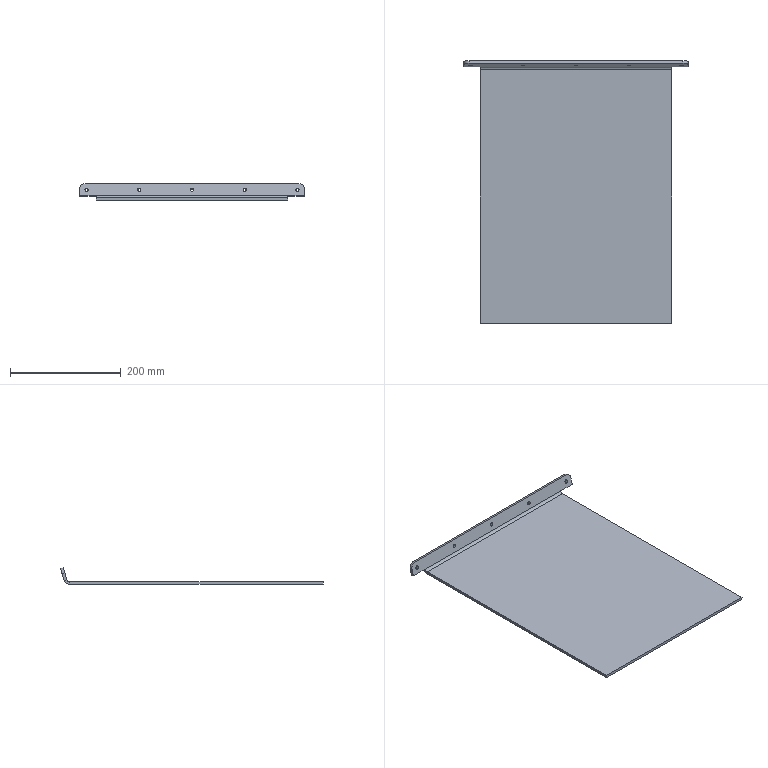Part | SolidWorks | features 3DProfileFeature 1, EdgeFlange 1, Fillet 1, FlatPattern 1, HoleWzd 1, SMBaseFlange 1, SheetMetal 1 | 1 solid | 38 faces | box 405 x 473.792 x 30.148 mm | volume 850700 mm3 | cylinder 14 | plane 14 | cone 10 | commonest cylinder face diameters 6 x10 20 x3 10 x1
STEP:
#1=CARTESIAN_POINT('',(-190.,237.073,15.005));
#2=VERTEX_POINT('',#1);
#3=CARTESIAN_POINT('',(-190.,238.832,20.741));
#4=VERTEX_POINT('',#3);
#5=CARTESIAN_POINT('',(-190.,237.952,17.873));
#6=DIRECTION('',(0.,0.9561,-0.2931));
#7=DIRECTION('',(0.,0.2931,0.9561));
#8=AXIS2_PLACEMENT_3D('',#5,#6,#7);
#9=CIRCLE('',#8,3.);
#10=EDGE_CURVE('',#2,#4,#9,.T.);
#11=ORIENTED_EDGE('',*,*,#10,.F.);
#12=CARTESIAN_POINT('',(-190.,237.09,14.974));
#13=VERTEX_POINT('',#12);
#14=CARTESIAN_POINT('',(-190.,237.09,14.974));
#15=DIRECTION('',(0.,0.4688,-0.8833));
#16=VECTOR('',#15,1000.);
#17=LINE('',#14,#16);
#18=EDGE_CURVE('',#2,#13,#17,.T.);
#19=ORIENTED_EDGE('',*,*,#18,.T.);
#20=CARTESIAN_POINT('',(-190.,238.863,20.758));
#21=VERTEX_POINT('',#20);
#22=CARTESIAN_POINT('',(-190.,237.976,17.866));
#23=DIRECTION('',(0.,0.9561,-0.2931));
#24=DIRECTION('',(0.,0.2931,0.9561));
#25=AXIS2_PLACEMENT_3D('',#22,#23,#24);
#26=CIRCLE('',#25,3.025);
#27=EDGE_CURVE('',#13,#21,#26,.T.);
#28=ORIENTED_EDGE('',*,*,#27,.T.);
#29=CARTESIAN_POINT('',(-190.,238.863,20.758));
#30=DIRECTION('',(0.,0.8833,0.4688));
#31=VECTOR('',#30,1000.);
#32=LINE('',#29,#31);
#33=EDGE_CURVE('',#4,#21,#32,.T.);
#34=ORIENTED_EDGE('',*,*,#33,.F.);
#35=EDGE_LOOP('',(#11,#19,#28,#34));
#36=FACE_OUTER_BOUND('',#35,.T.);
#37=CARTESIAN_POINT('',(-190.,237.976,17.866));
#38=DIRECTION('',(0.,0.9561,-0.2931));
#39=DIRECTION('',(0.,0.2931,0.9561));
#40=AXIS2_PLACEMENT_3D('',#37,#38,#39);
#41=CONICAL_SURFACE('',#40,3.025,0.7854);
#42=ADVANCED_FACE('',(#36),#41,.F.);
#43=CARTESIAN_POINT('',(-190.,232.317,16.463));
#44=VERTEX_POINT('',#43);
#45=CARTESIAN_POINT('',(-190.,234.075,22.199));
#46=VERTEX_POINT('',#45);
#47=CARTESIAN_POINT('',(-190.,233.196,19.331));
#48=DIRECTION('',(0.,0.9561,-0.2931));
#49=DIRECTION('',(0.,0.2931,0.9561));
#50=AXIS2_PLACEMENT_3D('',#47,#48,#49);
#51=CIRCLE('',#50,3.);
#52=EDGE_CURVE('',#44,#46,#51,.T.);
#53=ORIENTED_EDGE('',*,*,#52,.F.);
#54=CARTESIAN_POINT('',(-190.,237.097,14.998));
#55=DIRECTION('',(0.,0.9561,-0.2931));
#56=VECTOR('',#55,1000.);
#57=LINE('',#54,#56);
#58=EDGE_CURVE('',#44,#2,#57,.T.);
#59=ORIENTED_EDGE('',*,*,#58,.T.);
#60=ORIENTED_EDGE('',*,*,#10,.T.);
#61=CARTESIAN_POINT('',(-190.,238.855,20.734));
#62=DIRECTION('',(0.,0.9561,-0.2931));
#63=VECTOR('',#62,1000.);
#64=LINE('',#61,#63);
#65=EDGE_CURVE('',#46,#4,#64,.T.);
#66=ORIENTED_EDGE('',*,*,#65,.F.);
#67=EDGE_LOOP('',(#53,#59,#60,#66));
#68=FACE_OUTER_BOUND('',#67,.T.);
#69=CARTESIAN_POINT('',(-190.,237.976,17.866));
#70=DIRECTION('',(0.,0.9561,-0.2931));
#71=DIRECTION('',(0.,0.2931,0.9561));
#72=AXIS2_PLACEMENT_3D('',#69,#70,#71);
#73=CYLINDRICAL_SURFACE('',#72,3.);
#74=ADVANCED_FACE('',(#68),#73,.F.);
#75=CARTESIAN_POINT('',(-95.,237.073,15.005));
#76=VERTEX_POINT('',#75);
#77=CARTESIAN_POINT('',(-95.,238.832,20.741));
#78=VERTEX_POINT('',#77);
#79=CARTESIAN_POINT('',(-95.,237.952,17.873));
#80=DIRECTION('',(0.,0.9561,-0.2931));
#81=DIRECTION('',(0.,0.2931,0.9561));
#82=AXIS2_PLACEMENT_3D('',#79,#80,#81);
#83=CIRCLE('',#82,3.);
#84=EDGE_CURVE('',#76,#78,#83,.T.);
#85=ORIENTED_EDGE('',*,*,#84,.F.);
#86=CARTESIAN_POINT('',(-95.,237.09,14.974));
#87=VERTEX_POINT('',#86);
#88=CARTESIAN_POINT('',(-95.,237.09,14.974));
#89=DIRECTION('',(0.,0.4688,-0.8833));
#90=VECTOR('',#89,1000.);
#91=LINE('',#88,#90);
#92=EDGE_CURVE('',#76,#87,#91,.T.);
#93=ORIENTED_EDGE('',*,*,#92,.T.);
#94=CARTESIAN_POINT('',(-95.,238.863,20.758));
#95=VERTEX_POINT('',#94);
#96=CARTESIAN_POINT('',(-95.,237.976,17.866));
#97=DIRECTION('',(0.,0.9561,-0.2931));
#98=DIRECTION('',(0.,0.2931,0.9561));
#99=AXIS2_PLACEMENT_3D('',#96,#97,#98);
#100=CIRCLE('',#99,3.025);
#101=EDGE_CURVE('',#87,#95,#100,.T.);
#102=ORIENTED_EDGE('',*,*,#101,.T.);
#103=CARTESIAN_POINT('',(-95.,238.863,20.758));
#104=DIRECTION('',(0.,0.8833,0.4688));
#105=VECTOR('',#104,1000.);
#106=LINE('',#103,#105);
#107=EDGE_CURVE('',#78,#95,#106,.T.);
#108=ORIENTED_EDGE('',*,*,#107,.F.);
#109=EDGE_LOOP('',(#85,#93,#102,#108));
#110=FACE_OUTER_BOUND('',#109,.T.);
#111=CARTESIAN_POINT('',(-95.,237.976,17.866));
#112=DIRECTION('',(0.,0.9561,-0.2931));
#113=DIRECTION('',(0.,0.2931,0.9561));
#114=AXIS2_PLACEMENT_3D('',#111,#112,#113);
#115=CONICAL_SURFACE('',#114,3.025,0.7854);
#116=ADVANCED_FACE('',(#110),#115,.F.);
#117=CARTESIAN_POINT('',(-95.,232.317,16.463));
#118=VERTEX_POINT('',#117);
#119=CARTESIAN_POINT('',(-95.,234.075,22.199));
#120=VERTEX_POINT('',#119);
#121=CARTESIAN_POINT('',(-95.,233.196,19.331));
#122=DIRECTION('',(0.,0.9561,-0.2931));
#123=DIRECTION('',(0.,0.2931,0.9561));
#124=AXIS2_PLACEMENT_3D('',#121,#122,#123);
#125=CIRCLE('',#124,3.);
#126=EDGE_CURVE('',#118,#120,#125,.T.);
#127=ORIENTED_EDGE('',*,*,#126,.F.);
#128=CARTESIAN_POINT('',(-95.,237.097,14.998));
#129=DIRECTION('',(0.,0.9561,-0.2931));
#130=VECTOR('',#129,1000.);
#131=LINE('',#128,#130);
#132=EDGE_CURVE('',#118,#76,#131,.T.);
#133=ORIENTED_EDGE('',*,*,#132,.T.);
#134=ORIENTED_EDGE('',*,*,#84,.T.);
#135=CARTESIAN_POINT('',(-95.,238.855,20.734));
#136=DIRECTION('',(0.,0.9561,-0.2931));
#137=VECTOR('',#136,1000.);
#138=LINE('',#135,#137);
#139=EDGE_CURVE('',#120,#78,#138,.T.);
#140=ORIENTED_EDGE('',*,*,#139,.F.);
#141=EDGE_LOOP('',(#127,#133,#134,#140));
#142=FACE_OUTER_BOUND('',#141,.T.);
#143=CARTESIAN_POINT('',(-95.,237.976,17.866));
#144=DIRECTION('',(0.,0.9561,-0.2931));
#145=DIRECTION('',(0.,0.2931,0.9561));
#146=AXIS2_PLACEMENT_3D('',#143,#144,#145);
#147=CYLINDRICAL_SURFACE('',#146,3.);
#148=ADVANCED_FACE('',(#142),#147,.F.);
#149=CARTESIAN_POINT('',(0.,237.073,15.005));
#150=VERTEX_POINT('',#149);
#151=CARTESIAN_POINT('',(0.,238.832,20.741));
#152=VERTEX_POINT('',#151);
#153=CARTESIAN_POINT('',(0.,237.952,17.873));
#154=DIRECTION('',(0.,0.9561,-0.2931));
#155=DIRECTION('',(0.,0.2931,0.9561));
#156=AXIS2_PLACEMENT_3D('',#153,#154,#155);
#157=CIRCLE('',#156,3.);
#158=EDGE_CURVE('',#150,#152,#157,.T.);
#159=ORIENTED_EDGE('',*,*,#158,.F.);
#160=CARTESIAN_POINT('',(0.,237.09,14.974));
#161=VERTEX_POINT('',#160);
#162=CARTESIAN_POINT('',(0.,237.09,14.974));
#163=DIRECTION('',(0.,0.4688,-0.8833));
#164=VECTOR('',#163,1000.);
#165=LINE('',#162,#164);
#166=EDGE_CURVE('',#150,#161,#165,.T.);
#167=ORIENTED_EDGE('',*,*,#166,.T.);
#168=CARTESIAN_POINT('',(0.,238.863,20.758));
#169=VERTEX_POINT('',#168);
#170=CARTESIAN_POINT('',(0.,237.976,17.866));
#171=DIRECTION('',(0.,0.9561,-0.2931));
#172=DIRECTION('',(0.,0.2931,0.9561));
#173=AXIS2_PLACEMENT_3D('',#170,#171,#172);
#174=CIRCLE('',#173,3.025);
#175=EDGE_CURVE('',#161,#169,#174,.T.);
#176=ORIENTED_EDGE('',*,*,#175,.T.);
#177=CARTESIAN_POINT('',(0.,238.863,20.758));
#178=DIRECTION('',(0.,0.8833,0.4688));
#179=VECTOR('',#178,1000.);
#180=LINE('',#177,#179);
#181=EDGE_CURVE('',#152,#169,#180,.T.);
#182=ORIENTED_EDGE('',*,*,#181,.F.);
#183=EDGE_LOOP('',(#159,#167,#176,#182));
#184=FACE_OUTER_BOUND('',#183,.T.);
#185=CARTESIAN_POINT('',(0.,237.976,17.866));
#186=DIRECTION('',(0.,0.9561,-0.2931));
#187=DIRECTION('',(0.,0.2931,0.9561));
#188=AXIS2_PLACEMENT_3D('',#185,#186,#187);
#189=CONICAL_SURFACE('',#188,3.025,0.7854);
#190=ADVANCED_FACE('',(#184),#189,.F.);
#191=CARTESIAN_POINT('',(0.,232.317,16.463));
#192=VERTEX_POINT('',#191);
#193=CARTESIAN_POINT('',(0.,234.075,22.199));
#194=VERTEX_POINT('',#193);
#195=CARTESIAN_POINT('',(0.,233.196,19.331));
#196=DIRECTION('',(0.,0.9561,-0.2931));
#197=DIRECTION('',(0.,0.2931,0.9561));
#198=AXIS2_PLACEMENT_3D('',#195,#196,#197);
#199=CIRCLE('',#198,3.);
#200=EDGE_CURVE('',#192,#194,#199,.T.);
#201=ORIENTED_EDGE('',*,*,#200,.F.);
#202=CARTESIAN_POINT('',(0.,237.097,14.998));
#203=DIRECTION('',(0.,0.9561,-0.2931));
#204=VECTOR('',#203,1000.);
#205=LINE('',#202,#204);
#206=EDGE_CURVE('',#192,#150,#205,.T.);
#207=ORIENTED_EDGE('',*,*,#206,.T.);
#208=ORIENTED_EDGE('',*,*,#158,.T.);
#209=CARTESIAN_POINT('',(0.,238.855,20.734));
#210=DIRECTION('',(0.,0.9561,-0.2931));
#211=VECTOR('',#210,1000.);
#212=LINE('',#209,#211);
#213=EDGE_CURVE('',#194,#152,#212,.T.);
#214=ORIENTED_EDGE('',*,*,#213,.F.);
#215=EDGE_LOOP('',(#201,#207,#208,#214));
#216=FACE_OUTER_BOUND('',#215,.T.);
#217=CARTESIAN_POINT('',(0.,237.976,17.866));
#218=DIRECTION('',(0.,0.9561,-0.2931));
#219=DIRECTION('',(0.,0.2931,0.9561));
#220=AXIS2_PLACEMENT_3D('',#217,#218,#219);
#221=CYLINDRICAL_SURFACE('',#220,3.);
#222=ADVANCED_FACE('',(#216),#221,.F.);
#223=CARTESIAN_POINT('',(95.,237.073,15.005));
#224=VERTEX_POINT('',#223);
#225=CARTESIAN_POINT('',(95.,238.832,20.741));
#226=VERTEX_POINT('',#225);
#227=CARTESIAN_POINT('',(95.,237.952,17.873));
#228=DIRECTION('',(0.,0.9561,-0.2931));
#229=DIRECTION('',(0.,0.2931,0.9561));
#230=AXIS2_PLACEMENT_3D('',#227,#228,#229);
#231=CIRCLE('',#230,3.);
#232=EDGE_CURVE('',#224,#226,#231,.T.);
#233=ORIENTED_EDGE('',*,*,#232,.F.);
#234=CARTESIAN_POINT('',(95.,237.09,14.974));
#235=VERTEX_POINT('',#234);
#236=CARTESIAN_POINT('',(95.,237.09,14.974));
#237=DIRECTION('',(0.,0.4688,-0.8833));
#238=VECTOR('',#237,1000.);
#239=LINE('',#236,#238);
#240=EDGE_CURVE('',#224,#235,#239,.T.);
#241=ORIENTED_EDGE('',*,*,#240,.T.);
#242=CARTESIAN_POINT('',(95.,238.863,20.758));
#243=VERTEX_POINT('',#242);
#244=CARTESIAN_POINT('',(95.,237.976,17.866));
#245=DIRECTION('',(0.,0.9561,-0.2931));
#246=DIRECTION('',(0.,0.2931,0.9561));
#247=AXIS2_PLACEMENT_3D('',#244,#245,#246);
#248=CIRCLE('',#247,3.025);
#249=EDGE_CURVE('',#235,#243,#248,.T.);
#250=ORIENTED_EDGE('',*,*,#249,.T.);
#251=CARTESIAN_POINT('',(95.,238.863,20.758));
#252=DIRECTION('',(0.,0.8833,0.4688));
#253=VECTOR('',#252,1000.);
#254=LINE('',#251,#253);
#255=EDGE_CURVE('',#226,#243,#254,.T.);
#256=ORIENTED_EDGE('',*,*,#255,.F.);
#257=EDGE_LOOP('',(#233,#241,#250,#256));
#258=FACE_OUTER_BOUND('',#257,.T.);
#259=CARTESIAN_POINT('',(95.,237.976,17.866));
#260=DIRECTION('',(0.,0.9561,-0.2931));
#261=DIRECTION('',(0.,0.2931,0.9561));
#262=AXIS2_PLACEMENT_3D('',#259,#260,#261);
#263=CONICAL_SURFACE('',#262,3.025,0.7854);
#264=ADVANCED_FACE('',(#258),#263,.F.);
#265=CARTESIAN_POINT('',(95.,232.317,16.463));
#266=VERTEX_POINT('',#265);
#267=CARTESIAN_POINT('',(95.,234.075,22.199));
#268=VERTEX_POINT('',#267);
#269=CARTESIAN_POINT('',(95.,233.196,19.331));
#270=DIRECTION('',(0.,0.9561,-0.2931));
#271=DIRECTION('',(0.,0.2931,0.9561));
#272=AXIS2_PLACEMENT_3D('',#269,#270,#271);
#273=CIRCLE('',#272,3.);
#274=EDGE_CURVE('',#266,#268,#273,.T.);
#275=ORIENTED_EDGE('',*,*,#274,.F.);
#276=CARTESIAN_POINT('',(95.,237.097,14.998));
#277=DIRECTION('',(0.,0.9561,-0.2931));
#278=VECTOR('',#277,1000.);
#279=LINE('',#276,#278);
#280=EDGE_CURVE('',#266,#224,#279,.T.);
#281=ORIENTED_EDGE('',*,*,#280,.T.);
#282=ORIENTED_EDGE('',*,*,#232,.T.);
#283=CARTESIAN_POINT('',(95.,238.855,20.734));
#284=DIRECTION('',(0.,0.9561,-0.2931));
#285=VECTOR('',#284,1000.);
#286=LINE('',#283,#285);
#287=EDGE_CURVE('',#268,#226,#286,.T.);
#288=ORIENTED_EDGE('',*,*,#287,.F.);
#289=EDGE_LOOP('',(#275,#281,#282,#288));
#290=FACE_OUTER_BOUND('',#289,.T.);
#291=CARTESIAN_POINT('',(95.,237.976,17.866));
#292=DIRECTION('',(0.,0.9561,-0.2931));
#293=DIRECTION('',(0.,0.2931,0.9561));
#294=AXIS2_PLACEMENT_3D('',#291,#292,#293);
#295=CYLINDRICAL_SURFACE('',#294,3.);
#296=ADVANCED_FACE('',(#290),#295,.F.);
#297=CARTESIAN_POINT('',(190.,237.073,15.005));
#298=VERTEX_POINT('',#297);
#299=CARTESIAN_POINT('',(190.,238.832,20.741));
#300=VERTEX_POINT('',#299);
#301=CARTESIAN_POINT('',(190.,237.952,17.873));
#302=DIRECTION('',(0.,0.9561,-0.2931));
#303=DIRECTION('',(0.,0.2931,0.9561));
#304=AXIS2_PLACEMENT_3D('',#301,#302,#303);
#305=CIRCLE('',#304,3.);
#306=EDGE_CURVE('',#298,#300,#305,.T.);
#307=ORIENTED_EDGE('',*,*,#306,.F.);
#308=CARTESIAN_POINT('',(190.,237.09,14.974));
#309=VERTEX_POINT('',#308);
#310=CARTESIAN_POINT('',(190.,237.09,14.974));
#311=DIRECTION('',(0.,0.4688,-0.8833));
#312=VECTOR('',#311,1000.);
#313=LINE('',#310,#312);
#314=EDGE_CURVE('',#298,#309,#313,.T.);
#315=ORIENTED_EDGE('',*,*,#314,.T.);
#316=CARTESIAN_POINT('',(190.,238.863,20.758));
#317=VERTEX_POINT('',#316);
#318=CARTESIAN_POINT('',(190.,237.976,17.866));
#319=DIRECTION('',(0.,0.9561,-0.2931));
#320=DIRECTION('',(0.,0.2931,0.9561));
#321=AXIS2_PLACEMENT_3D('',#318,#319,#320);
#322=CIRCLE('',#321,3.025);
#323=EDGE_CURVE('',#309,#317,#322,.T.);
#324=ORIENTED_EDGE('',*,*,#323,.T.);
#325=CARTESIAN_POINT('',(190.,238.863,20.758));
#326=DIRECTION('',(0.,0.8833,0.4688));
#327=VECTOR('',#326,1000.);
#328=LINE('',#325,#327);
#329=EDGE_CURVE('',#300,#317,#328,.T.);
#330=ORIENTED_EDGE('',*,*,#329,.F.);
#331=EDGE_LOOP('',(#307,#315,#324,#330));
#332=FACE_OUTER_BOUND('',#331,.T.);
#333=CARTESIAN_POINT('',(190.,237.976,17.866));
#334=DIRECTION('',(0.,0.9561,-0.2931));
#335=DIRECTION('',(0.,0.2931,0.9561));
#336=AXIS2_PLACEMENT_3D('',#333,#334,#335);
#337=CONICAL_SURFACE('',#336,3.025,0.7854);
#338=ADVANCED_FACE('',(#332),#337,.F.);
#339=CARTESIAN_POINT('',(190.,232.317,16.463));
#340=VERTEX_POINT('',#339);
#341=CARTESIAN_POINT('',(190.,234.075,22.199));
#342=VERTEX_POINT('',#341);
#343=CARTESIAN_POINT('',(190.,233.196,19.331));
#344=DIRECTION('',(0.,0.9561,-0.2931));
#345=DIRECTION('',(0.,0.2931,0.9561));
#346=AXIS2_PLACEMENT_3D('',#343,#344,#345);
#347=CIRCLE('',#346,3.);
#348=EDGE_CURVE('',#340,#342,#347,.T.);
#349=ORIENTED_EDGE('',*,*,#348,.F.);
#350=CARTESIAN_POINT('',(190.,237.097,14.998));
#351=DIRECTION('',(0.,0.9561,-0.2931));
#352=VECTOR('',#351,1000.);
#353=LINE('',#350,#352);
#354=EDGE_CURVE('',#340,#298,#353,.T.);
#355=ORIENTED_EDGE('',*,*,#354,.T.);
#356=ORIENTED_EDGE('',*,*,#306,.T.);
#357=CARTESIAN_POINT('',(190.,238.855,20.734));
#358=DIRECTION('',(0.,0.9561,-0.2931));
#359=VECTOR('',#358,1000.);
#360=LINE('',#357,#359);
#361=EDGE_CURVE('',#342,#300,#360,.T.);
#362=ORIENTED_EDGE('',*,*,#361,.F.);
#363=EDGE_LOOP('',(#349,#355,#356,#362));
#364=FACE_OUTER_BOUND('',#363,.T.);
#365=CARTESIAN_POINT('',(190.,237.976,17.866));
#366=DIRECTION('',(0.,0.9561,-0.2931));
#367=DIRECTION('',(0.,0.2931,0.9561));
#368=AXIS2_PLACEMENT_3D('',#365,#366,#367);
#369=CYLINDRICAL_SURFACE('',#368,3.);
#370=ADVANCED_FACE('',(#364),#369,.F.);
#371=CARTESIAN_POINT('',(172.5,225.106,5.));
#372=VERTEX_POINT('',#371);
#373=CARTESIAN_POINT('',(172.5,225.106,0.));
#374=VERTEX_POINT('',#373);
#375=CARTESIAN_POINT('',(172.5,225.106,5.));
#376=DIRECTION('',(0.,0.,-1.));
#377=VECTOR('',#376,1000.);
#378=LINE('',#375,#377);
#379=EDGE_CURVE('',#372,#374,#378,.T.);
#380=ORIENTED_EDGE('',*,*,#379,.F.);
#381=CARTESIAN_POINT('',(172.5,-232.5,5.));
#382=VERTEX_POINT('',#381);
#383=CARTESIAN_POINT('',(172.5,232.5,5.));
#384=DIRECTION('',(0.,1.,0.));
#385=VECTOR('',#384,1000.);
#386=LINE('',#383,#385);
#387=EDGE_CURVE('',#382,#372,#386,.T.);
#388=ORIENTED_EDGE('',*,*,#387,.F.);
#389=CARTESIAN_POINT('',(172.5,-232.5,0.));
#390=VERTEX_POINT('',#389);
#391=CARTESIAN_POINT('',(172.5,-232.5,5.));
#392=DIRECTION('',(0.,0.,-1.));
#393=VECTOR('',#392,1000.);
#394=LINE('',#391,#393);
#395=EDGE_CURVE('',#382,#390,#394,.T.);
#396=ORIENTED_EDGE('',*,*,#395,.T.);
#397=CARTESIAN_POINT('',(172.5,232.5,0.));
#398=DIRECTION('',(0.,1.,0.));
#399=VECTOR('',#398,1000.);
#400=LINE('',#397,#399);
#401=EDGE_CURVE('',#390,#374,#400,.T.);
#402=ORIENTED_EDGE('',*,*,#401,.T.);
#403=EDGE_LOOP('',(#380,#388,#396,#402));
#404=FACE_OUTER_BOUND('',#403,.T.);
#405=CARTESIAN_POINT('',(172.5,232.5,5.));
#406=DIRECTION('',(-1.,0.,0.));
#407=DIRECTION('',(0.,-1.,0.));
#408=AXIS2_PLACEMENT_3D('',#405,#406,#407);
#409=PLANE('',#408);
#410=ADVANCED_FACE('',(#404),#409,.F.);
#411=CARTESIAN_POINT('',(-172.5,225.106,5.));
#412=VERTEX_POINT('',#411);
#413=CARTESIAN_POINT('',(-172.5,225.106,0.));
#414=VERTEX_POINT('',#413);
#415=CARTESIAN_POINT('',(-172.5,225.106,5.));
#416=DIRECTION('',(0.,0.,-1.));
#417=VECTOR('',#416,1000.);
#418=LINE('',#415,#417);
#419=EDGE_CURVE('',#412,#414,#418,.T.);
#420=ORIENTED_EDGE('',*,*,#419,.T.);
#421=CARTESIAN_POINT('',(-172.5,-232.5,0.));
#422=VERTEX_POINT('',#421);
#423=CARTESIAN_POINT('',(-172.5,232.5,0.));
#424=DIRECTION('',(0.,-1.,0.));
#425=VECTOR('',#424,1000.);
#426=LINE('',#423,#425);
#427=EDGE_CURVE('',#414,#422,#426,.T.);
#428=ORIENTED_EDGE('',*,*,#427,.T.);
#429=CARTESIAN_POINT('',(-172.5,-232.5,5.));
#430=VERTEX_POINT('',#429);
#431=CARTESIAN_POINT('',(-172.5,-232.5,5.));
#432=DIRECTION('',(0.,0.,-1.));
#433=VECTOR('',#432,1000.);
#434=LINE('',#431,#433);
#435=EDGE_CURVE('',#430,#422,#434,.T.);
#436=ORIENTED_EDGE('',*,*,#435,.F.);
#437=CARTESIAN_POINT('',(-172.5,232.5,5.));
#438=DIRECTION('',(0.,-1.,0.));
#439=VECTOR('',#438,1000.);
#440=LINE('',#437,#439);
#441=EDGE_CURVE('',#412,#430,#440,.T.);
#442=ORIENTED_EDGE('',*,*,#441,.F.);
#443=EDGE_LOOP('',(#420,#428,#436,#442));
#444=FACE_OUTER_BOUND('',#443,.T.);
#445=CARTESIAN_POINT('',(-172.5,232.5,5.));
#446=DIRECTION('',(1.,0.,0.));
#447=DIRECTION('',(0.,1.,0.));
#448=AXIS2_PLACEMENT_3D('',#445,#446,#447);
#449=PLANE('',#448);
#450=ADVANCED_FACE('',(#444),#449,.F.);
#451=ORIENTED_EDGE('',*,*,#387,.T.);
#452=CARTESIAN_POINT('',(-172.5,225.106,5.));
#453=DIRECTION('',(1.,0.,0.));
#454=VECTOR('',#453,1000.);
#455=LINE('',#452,#454);
#456=EDGE_CURVE('',#412,#372,#455,.T.);
#457=ORIENTED_EDGE('',*,*,#456,.F.);
#458=ORIENTED_EDGE('',*,*,#441,.T.);
#459=CARTESIAN_POINT('',(-172.5,-232.5,5.));
#460=DIRECTION('',(1.,0.,0.));
#461=VECTOR('',#460,1000.);
#462=LINE('',#459,#461);
#463=EDGE_CURVE('',#430,#382,#462,.T.);
#464=ORIENTED_EDGE('',*,*,#463,.T.);
#465=EDGE_LOOP('',(#451,#457,#458,#464));
#466=FACE_OUTER_BOUND('',#465,.T.);
#467=CARTESIAN_POINT('',(0.,0.,5.));
#468=DIRECTION('',(0.,0.,1.));
#469=DIRECTION('',(1.,0.,0.));
#470=AXIS2_PLACEMENT_3D('',#467,#468,#469);
#471=PLANE('',#470);
#472=ADVANCED_FACE('',(#466),#471,.T.);
#473=CARTESIAN_POINT('',(-172.5,225.106,0.));
#474=DIRECTION('',(1.,0.,0.));
#475=VECTOR('',#474,1000.);
#476=LINE('',#473,#475);
#477=EDGE_CURVE('',#414,#374,#476,.T.);
#478=ORIENTED_EDGE('',*,*,#477,.T.);
#479=ORIENTED_EDGE('',*,*,#401,.F.);
#480=CARTESIAN_POINT('',(-172.5,-232.5,0.));
#481=DIRECTION('',(1.,0.,0.));
#482=VECTOR('',#481,1000.);
#483=LINE('',#480,#482);
#484=EDGE_CURVE('',#422,#390,#483,.T.);
#485=ORIENTED_EDGE('',*,*,#484,.F.);
#486=ORIENTED_EDGE('',*,*,#427,.F.);
#487=EDGE_LOOP('',(#478,#479,#485,#486));
#488=FACE_OUTER_BOUND('',#487,.T.);
#489=CARTESIAN_POINT('',(0.,0.,0.));
#490=DIRECTION('',(0.,0.,1.));
#491=DIRECTION('',(1.,0.,0.));
#492=AXIS2_PLACEMENT_3D('',#489,#490,#491);
#493=PLANE('',#492);
#494=ADVANCED_FACE('',(#488),#493,.F.);
#495=ORIENTED_EDGE('',*,*,#484,.T.);
#496=ORIENTED_EDGE('',*,*,#395,.F.);
#497=ORIENTED_EDGE('',*,*,#463,.F.);
#498=ORIENTED_EDGE('',*,*,#435,.T.);
#499=EDGE_LOOP('',(#495,#496,#497,#498));
#500=FACE_OUTER_BOUND('',#499,.T.);
#501=CARTESIAN_POINT('',(-172.5,-232.5,5.));
#502=DIRECTION('',(0.,1.,0.));
#503=DIRECTION('',(0.,0.,1.));
#504=AXIS2_PLACEMENT_3D('',#501,#502,#503);
#505=PLANE('',#504);
#506=ADVANCED_FACE('',(#500),#505,.F.);
#507=CARTESIAN_POINT('',(172.5,229.886,8.535));
#508=VERTEX_POINT('',#507);
#509=CARTESIAN_POINT('',(172.5,234.667,7.069));
#510=VERTEX_POINT('',#509);
#511=CARTESIAN_POINT('',(172.5,229.886,8.535));
#512=DIRECTION('',(0.,0.9561,-0.2931));
#513=VECTOR('',#512,1000.);
#514=LINE('',#511,#513);
#515=EDGE_CURVE('',#508,#510,#514,.T.);
#516=ORIENTED_EDGE('',*,*,#515,.F.);
#517=CARTESIAN_POINT('',(172.5,225.106,10.));
#518=DIRECTION('',(1.,0.,0.));
#519=DIRECTION('',(0.,0.,1.));
#520=AXIS2_PLACEMENT_3D('',#517,#518,#519);
#521=CIRCLE('',#520,5.);
#522=EDGE_CURVE('',#372,#508,#521,.T.);
#523=ORIENTED_EDGE('',*,*,#522,.F.);
#524=ORIENTED_EDGE('',*,*,#379,.T.);
#525=CARTESIAN_POINT('',(172.5,225.106,10.));
#526=DIRECTION('',(1.,0.,0.));
#527=DIRECTION('',(0.,0.,1.));
#528=AXIS2_PLACEMENT_3D('',#525,#526,#527);
#529=CIRCLE('',#528,10.);
#530=EDGE_CURVE('',#374,#510,#529,.T.);
#531=ORIENTED_EDGE('',*,*,#530,.T.);
#532=EDGE_LOOP('',(#516,#523,#524,#531));
#533=FACE_OUTER_BOUND('',#532,.T.);
#534=CARTESIAN_POINT('',(172.5,225.106,10.));
#535=DIRECTION('',(1.,0.,0.));
#536=DIRECTION('',(0.,0.,-1.));
#537=AXIS2_PLACEMENT_3D('',#534,#535,#536);
#538=PLANE('',#537);
#539=ADVANCED_FACE('',(#533),#538,.T.);
#540=CARTESIAN_POINT('',(-172.5,229.886,8.535));
#541=VERTEX_POINT('',#540);
#542=CARTESIAN_POINT('',(-172.5,225.106,10.));
#543=DIRECTION('',(-1.,0.,0.));
#544=DIRECTION('',(0.,0.,1.));
#545=AXIS2_PLACEMENT_3D('',#542,#543,#544);
#546=CIRCLE('',#545,5.);
#547=EDGE_CURVE('',#541,#412,#546,.T.);
#548=ORIENTED_EDGE('',*,*,#547,.F.);
#549=CARTESIAN_POINT('',(-172.5,234.667,7.069));
#550=VERTEX_POINT('',#549);
#551=CARTESIAN_POINT('',(-172.5,229.886,8.535));
#552=DIRECTION('',(0.,0.9561,-0.2931));
#553=VECTOR('',#552,1000.);
#554=LINE('',#551,#553);
#555=EDGE_CURVE('',#541,#550,#554,.T.);
#556=ORIENTED_EDGE('',*,*,#555,.T.);
#557=CARTESIAN_POINT('',(-172.5,225.106,10.));
#558=DIRECTION('',(-1.,0.,0.));
#559=DIRECTION('',(0.,0.,1.));
#560=AXIS2_PLACEMENT_3D('',#557,#558,#559);
#561=CIRCLE('',#560,10.);
#562=EDGE_CURVE('',#550,#414,#561,.T.);
#563=ORIENTED_EDGE('',*,*,#562,.T.);
#564=ORIENTED_EDGE('',*,*,#419,.F.);
#565=EDGE_LOOP('',(#548,#556,#563,#564));
#566=FACE_OUTER_BOUND('',#565,.T.);
#567=CARTESIAN_POINT('',(-172.5,225.106,10.));
#568=DIRECTION('',(1.,0.,0.));
#569=DIRECTION('',(0.,0.,-1.));
#570=AXIS2_PLACEMENT_3D('',#567,#568,#569);
#571=PLANE('',#570);
#572=ADVANCED_FACE('',(#566),#571,.F.);
#573=ORIENTED_EDGE('',*,*,#477,.F.);
#574=ORIENTED_EDGE('',*,*,#562,.F.);
#575=CARTESIAN_POINT('',(-172.5,234.667,7.069));
#576=DIRECTION('',(-1.,0.,0.));
#577=VECTOR('',#576,1000.);
#578=LINE('',#575,#577);
#579=EDGE_CURVE('',#510,#550,#578,.T.);
#580=ORIENTED_EDGE('',*,*,#579,.F.);
#581=ORIENTED_EDGE('',*,*,#530,.F.);
#582=EDGE_LOOP('',(#573,#574,#580,#581));
#583=FACE_OUTER_BOUND('',#582,.T.);
#584=CARTESIAN_POINT('',(-172.5,225.106,10.));
#585=DIRECTION('',(-1.,0.,0.));
#586=DIRECTION('',(0.,0.9561,-0.2931));
#587=AXIS2_PLACEMENT_3D('',#584,#585,#586);
#588=CYLINDRICAL_SURFACE('',#587,10.);
#589=ADVANCED_FACE('',(#583),#588,.T.);
#590=ORIENTED_EDGE('',*,*,#456,.T.);
#591=ORIENTED_EDGE('',*,*,#522,.T.);
#592=CARTESIAN_POINT('',(-172.5,229.886,8.535));
#593=DIRECTION('',(-1.,0.,0.));
#594=VECTOR('',#593,1000.);
#595=LINE('',#592,#594);
#596=EDGE_CURVE('',#508,#541,#595,.T.);
#597=ORIENTED_EDGE('',*,*,#596,.T.);
#598=ORIENTED_EDGE('',*,*,#547,.T.);
#599=EDGE_LOOP('',(#590,#591,#597,#598));
#600=FACE_OUTER_BOUND('',#599,.T.);
#601=CARTESIAN_POINT('',(-172.5,225.106,10.));
#602=DIRECTION('',(-1.,0.,0.));
#603=DIRECTION('',(0.,0.9561,-0.2931));
#604=AXIS2_PLACEMENT_3D('',#601,#602,#603);
#605=CYLINDRICAL_SURFACE('',#604,5.);
#606=ADVANCED_FACE('',(#600),#605,.F.);
#607=ORIENTED_EDGE('',*,*,#555,.F.);
#608=CARTESIAN_POINT('',(-202.5,229.886,8.535));
#609=VERTEX_POINT('',#608);
#610=CARTESIAN_POINT('',(202.5,229.886,8.535));
#611=DIRECTION('',(-1.,0.,0.));
#612=VECTOR('',#611,1000.);
#613=LINE('',#610,#612);
#614=EDGE_CURVE('',#541,#609,#613,.T.);
#615=ORIENTED_EDGE('',*,*,#614,.T.);
#616=CARTESIAN_POINT('',(-202.5,234.667,7.069));
#617=VERTEX_POINT('',#616);
#618=CARTESIAN_POINT('',(-202.5,229.886,8.535));
#619=DIRECTION('',(0.,0.9561,-0.2931));
#620=VECTOR('',#619,1000.);
#621=LINE('',#618,#620);
#622=EDGE_CURVE('',#609,#617,#621,.T.);
#623=ORIENTED_EDGE('',*,*,#622,.T.);
#624=CARTESIAN_POINT('',(0.,234.667,7.069));
#625=DIRECTION('',(-1.,0.,0.));
#626=VECTOR('',#625,1000.);
#627=LINE('',#624,#626);
#628=EDGE_CURVE('',#550,#617,#627,.T.);
#629=ORIENTED_EDGE('',*,*,#628,.F.);
#630=EDGE_LOOP('',(#607,#615,#623,#629));
#631=FACE_OUTER_BOUND('',#630,.T.);
#632=CARTESIAN_POINT('',(202.5,229.886,8.535));
#633=DIRECTION('',(0.,-0.2931,-0.9561));
#634=DIRECTION('',(0.,0.9561,-0.2931));
#635=AXIS2_PLACEMENT_3D('',#632,#633,#634);
#636=PLANE('',#635);
#637=ADVANCED_FACE('',(#631),#636,.T.);
#638=CARTESIAN_POINT('',(-202.5,233.581,20.587));
#639=VERTEX_POINT('',#638);
#640=CARTESIAN_POINT('',(-202.5,207.434,-64.716));
#641=DIRECTION('',(0.,-0.2931,-0.9561));
#642=VECTOR('',#641,1000.);
#643=LINE('',#640,#642);
#644=EDGE_CURVE('',#639,#609,#643,.T.);
#645=ORIENTED_EDGE('',*,*,#644,.F.);
#646=CARTESIAN_POINT('',(-202.5,238.361,19.122));
#647=VERTEX_POINT('',#646);
#648=CARTESIAN_POINT('',(-202.5,238.361,19.122));
#649=DIRECTION('',(0.,0.9561,-0.2931));
#650=VECTOR('',#649,1000.);
#651=LINE('',#648,#650);
#652=EDGE_CURVE('',#639,#647,#651,.T.);
#653=ORIENTED_EDGE('',*,*,#652,.T.);
#654=CARTESIAN_POINT('',(-202.5,233.583,3.535));
#655=DIRECTION('',(0.,-0.2931,-0.9561));
#656=VECTOR('',#655,1000.);
#657=LINE('',#654,#656);
#658=EDGE_CURVE('',#647,#617,#657,.T.);
#659=ORIENTED_EDGE('',*,*,#658,.T.);
#660=ORIENTED_EDGE('',*,*,#622,.F.);
#661=EDGE_LOOP('',(#645,#653,#659,#660));
#662=FACE_OUTER_BOUND('',#661,.T.);
#663=CARTESIAN_POINT('',(-202.5,233.583,3.535));
#664=DIRECTION('',(-1.,0.,0.));
#665=DIRECTION('',(0.,0.,1.));
#666=AXIS2_PLACEMENT_3D('',#663,#664,#665);
#667=PLANE('',#666);
#668=ADVANCED_FACE('',(#662),#667,.T.);
#669=CARTESIAN_POINT('',(202.5,234.667,7.069));
#670=VERTEX_POINT('',#669);
#671=CARTESIAN_POINT('',(202.5,238.361,19.122));
#672=VERTEX_POINT('',#671);
#673=CARTESIAN_POINT('',(202.5,241.292,28.683));
#674=DIRECTION('',(0.,0.2931,0.9561));
#675=VECTOR('',#674,1000.);
#676=LINE('',#673,#675);
#677=EDGE_CURVE('',#670,#672,#676,.T.);
#678=ORIENTED_EDGE('',*,*,#677,.T.);
#679=CARTESIAN_POINT('',(202.5,233.581,20.587));
#680=VERTEX_POINT('',#679);
#681=CARTESIAN_POINT('',(202.5,238.361,19.122));
#682=DIRECTION('',(0.,-0.9561,0.2931));
#683=VECTOR('',#682,1000.);
#684=LINE('',#681,#683);
#685=EDGE_CURVE('',#672,#680,#684,.T.);
#686=ORIENTED_EDGE('',*,*,#685,.T.);
#687=CARTESIAN_POINT('',(202.5,229.886,8.535));
#688=VERTEX_POINT('',#687);
#689=CARTESIAN_POINT('',(202.5,207.434,-64.716));
#690=DIRECTION('',(0.,0.2931,0.9561));
#691=VECTOR('',#690,1000.);
#692=LINE('',#689,#691);
#693=EDGE_CURVE('',#688,#680,#692,.T.);
#694=ORIENTED_EDGE('',*,*,#693,.F.);
#695=CARTESIAN_POINT('',(202.5,234.667,7.069));
#696=DIRECTION('',(0.,0.9561,-0.2931));
#697=VECTOR('',#696,1000.);
#698=LINE('',#695,#697);
#699=EDGE_CURVE('',#688,#670,#698,.T.);
#700=ORIENTED_EDGE('',*,*,#699,.T.);
#701=EDGE_LOOP('',(#678,#686,#694,#700));
#702=FACE_OUTER_BOUND('',#701,.T.);
#703=CARTESIAN_POINT('',(202.5,241.292,28.683));
#704=DIRECTION('',(1.,0.,0.));
#705=DIRECTION('',(0.,0.,-1.));
#706=AXIS2_PLACEMENT_3D('',#703,#704,#705);
#707=PLANE('',#706);
#708=ADVANCED_FACE('',(#702),#707,.T.);
#709=CARTESIAN_POINT('',(-190.,237.976,17.866));
#710=DIRECTION('',(0.,0.9561,-0.2931));
#711=DIRECTION('',(0.,0.2931,0.9561));
#712=AXIS2_PLACEMENT_3D('',#709,#710,#711);
#713=CIRCLE('',#712,3.025);
#714=EDGE_CURVE('',#21,#13,#713,.T.);
#715=ORIENTED_EDGE('',*,*,#714,.F.);
#716=ORIENTED_EDGE('',*,*,#27,.F.);
#717=EDGE_LOOP('',(#715,#716));
#718=FACE_BOUND('',#717,.T.);
#719=CARTESIAN_POINT('',(-95.,237.976,17.866));
#720=DIRECTION('',(0.,0.9561,-0.2931));
#721=DIRECTION('',(0.,0.2931,0.9561));
#722=AXIS2_PLACEMENT_3D('',#719,#720,#721);
#723=CIRCLE('',#722,3.025);
#724=EDGE_CURVE('',#95,#87,#723,.T.);
#725=ORIENTED_EDGE('',*,*,#724,.F.);
#726=ORIENTED_EDGE('',*,*,#101,.F.);
#727=EDGE_LOOP('',(#725,#726));
#728=FACE_BOUND('',#727,.T.);
#729=CARTESIAN_POINT('',(0.,237.976,17.866));
#730=DIRECTION('',(0.,0.9561,-0.2931));
#731=DIRECTION('',(0.,0.2931,0.9561));
#732=AXIS2_PLACEMENT_3D('',#729,#730,#731);
#733=CIRCLE('',#732,3.025);
#734=EDGE_CURVE('',#169,#161,#733,.T.);
#735=ORIENTED_EDGE('',*,*,#734,.F.);
#736=ORIENTED_EDGE('',*,*,#175,.F.);
#737=EDGE_LOOP('',(#735,#736));
#738=FACE_BOUND('',#737,.T.);
#739=CARTESIAN_POINT('',(95.,237.976,17.866));
#740=DIRECTION('',(0.,0.9561,-0.2931));
#741=DIRECTION('',(0.,0.2931,0.9561));
#742=AXIS2_PLACEMENT_3D('',#739,#740,#741);
#743=CIRCLE('',#742,3.025);
#744=EDGE_CURVE('',#243,#235,#743,.T.);
#745=ORIENTED_EDGE('',*,*,#744,.F.);
#746=ORIENTED_EDGE('',*,*,#249,.F.);
#747=EDGE_LOOP('',(#745,#746));
#748=FACE_BOUND('',#747,.T.);
#749=CARTESIAN_POINT('',(190.,237.976,17.866));
#750=DIRECTION('',(0.,0.9561,-0.2931));
#751=DIRECTION('',(0.,0.2931,0.9561));
#752=AXIS2_PLACEMENT_3D('',#749,#750,#751);
#753=CIRCLE('',#752,3.025);
#754=EDGE_CURVE('',#317,#309,#753,.T.);
#755=ORIENTED_EDGE('',*,*,#754,.F.);
#756=ORIENTED_EDGE('',*,*,#323,.F.);
#757=EDGE_LOOP('',(#755,#756));
#758=FACE_BOUND('',#757,.T.);
#759=ORIENTED_EDGE('',*,*,#658,.F.);
#760=CARTESIAN_POINT('',(-192.5,241.292,28.683));
#761=VERTEX_POINT('',#760);
#762=CARTESIAN_POINT('',(-192.5,238.361,19.122));
#763=DIRECTION('',(0.,0.9561,-0.2931));
#764=DIRECTION('',(0.,0.2931,0.9561));
#765=AXIS2_PLACEMENT_3D('',#762,#763,#764);
#766=CIRCLE('',#765,10.);
#767=EDGE_CURVE('',#647,#761,#766,.T.);
#768=ORIENTED_EDGE('',*,*,#767,.T.);
#769=CARTESIAN_POINT('',(192.5,241.292,28.683));
#770=VERTEX_POINT('',#769);
#771=CARTESIAN_POINT('',(-202.5,241.292,28.683));
#772=DIRECTION('',(-1.,0.,0.));
#773=VECTOR('',#772,1000.);
#774=LINE('',#771,#773);
#775=EDGE_CURVE('',#770,#761,#774,.T.);
#776=ORIENTED_EDGE('',*,*,#775,.F.);
#777=CARTESIAN_POINT('',(192.5,238.361,19.122));
#778=DIRECTION('',(0.,0.9561,-0.2931));
#779=DIRECTION('',(0.,0.2931,0.9561));
#780=AXIS2_PLACEMENT_3D('',#777,#778,#779);
#781=CIRCLE('',#780,10.);
#782=EDGE_CURVE('',#770,#672,#781,.T.);
#783=ORIENTED_EDGE('',*,*,#782,.T.);
#784=ORIENTED_EDGE('',*,*,#677,.F.);
#785=CARTESIAN_POINT('',(0.,234.667,7.069));
#786=DIRECTION('',(-1.,0.,0.));
#787=VECTOR('',#786,1000.);
#788=LINE('',#785,#787);
#789=EDGE_CURVE('',#670,#510,#788,.T.);
#790=ORIENTED_EDGE('',*,*,#789,.T.);
#791=ORIENTED_EDGE('',*,*,#579,.T.);
#792=ORIENTED_EDGE('',*,*,#628,.T.);
#793=EDGE_LOOP('',(#759,#768,#776,#783,#784,#790,#791,#792));
#794=FACE_OUTER_BOUND('',#793,.T.);
#795=CARTESIAN_POINT('',(0.,212.214,-66.181));
#796=DIRECTION('',(0.,0.9561,-0.2931));
#797=DIRECTION('',(0.,0.2931,0.9561));
#798=AXIS2_PLACEMENT_3D('',#795,#796,#797);
#799=PLANE('',#798);
#800=ADVANCED_FACE('',(#718,#728,#738,#748,#758,#794),#799,.T.);
#801=CARTESIAN_POINT('',(-190.,233.196,19.331));
#802=DIRECTION('',(0.,0.9561,-0.2931));
#803=DIRECTION('',(0.,0.2931,0.9561));
#804=AXIS2_PLACEMENT_3D('',#801,#802,#803);
#805=CIRCLE('',#804,3.);
#806=EDGE_CURVE('',#46,#44,#805,.T.);
#807=ORIENTED_EDGE('',*,*,#806,.T.);
#808=ORIENTED_EDGE('',*,*,#52,.T.);
#809=EDGE_LOOP('',(#807,#808));
#810=FACE_BOUND('',#809,.T.);
#811=CARTESIAN_POINT('',(-95.,233.196,19.331));
#812=DIRECTION('',(0.,0.9561,-0.2931));
#813=DIRECTION('',(0.,0.2931,0.9561));
#814=AXIS2_PLACEMENT_3D('',#811,#812,#813);
#815=CIRCLE('',#814,3.);
#816=EDGE_CURVE('',#120,#118,#815,.T.);
#817=ORIENTED_EDGE('',*,*,#816,.T.);
#818=ORIENTED_EDGE('',*,*,#126,.T.);
#819=EDGE_LOOP('',(#817,#818));
#820=FACE_BOUND('',#819,.T.);
#821=CARTESIAN_POINT('',(0.,233.196,19.331));
#822=DIRECTION('',(0.,0.9561,-0.2931));
#823=DIRECTION('',(0.,0.2931,0.9561));
#824=AXIS2_PLACEMENT_3D('',#821,#822,#823);
#825=CIRCLE('',#824,3.);
#826=EDGE_CURVE('',#194,#192,#825,.T.);
#827=ORIENTED_EDGE('',*,*,#826,.T.);
#828=ORIENTED_EDGE('',*,*,#200,.T.);
#829=EDGE_LOOP('',(#827,#828));
#830=FACE_BOUND('',#829,.T.);
#831=CARTESIAN_POINT('',(95.,233.196,19.331));
#832=DIRECTION('',(0.,0.9561,-0.2931));
#833=DIRECTION('',(0.,0.2931,0.9561));
#834=AXIS2_PLACEMENT_3D('',#831,#832,#833);
#835=CIRCLE('',#834,3.);
#836=EDGE_CURVE('',#268,#266,#835,.T.);
#837=ORIENTED_EDGE('',*,*,#836,.T.);
#838=ORIENTED_EDGE('',*,*,#274,.T.);
#839=EDGE_LOOP('',(#837,#838));
#840=FACE_BOUND('',#839,.T.);
#841=CARTESIAN_POINT('',(190.,233.196,19.331));
#842=DIRECTION('',(0.,0.9561,-0.2931));
#843=DIRECTION('',(0.,0.2931,0.9561));
#844=AXIS2_PLACEMENT_3D('',#841,#842,#843);
#845=CIRCLE('',#844,3.);
#846=EDGE_CURVE('',#342,#340,#845,.T.);
#847=ORIENTED_EDGE('',*,*,#846,.T.);
#848=ORIENTED_EDGE('',*,*,#348,.T.);
#849=EDGE_LOOP('',(#847,#848));
#850=FACE_BOUND('',#849,.T.);
#851=CARTESIAN_POINT('',(192.5,236.511,30.148));
#852=VERTEX_POINT('',#851);
#853=CARTESIAN_POINT('',(-192.5,236.511,30.148));
#854=VERTEX_POINT('',#853);
#855=CARTESIAN_POINT('',(0.,236.511,30.148));
#856=DIRECTION('',(-1.,0.,0.));
#857=VECTOR('',#856,1000.);
#858=LINE('',#855,#857);
#859=EDGE_CURVE('',#852,#854,#858,.T.);
#860=ORIENTED_EDGE('',*,*,#859,.T.);
#861=CARTESIAN_POINT('',(-192.5,233.581,20.587));
#862=DIRECTION('',(0.,-0.9561,0.2931));
#863=DIRECTION('',(0.,0.2931,0.9561));
#864=AXIS2_PLACEMENT_3D('',#861,#862,#863);
#865=CIRCLE('',#864,10.);
#866=EDGE_CURVE('',#854,#639,#865,.T.);
#867=ORIENTED_EDGE('',*,*,#866,.T.);
#868=ORIENTED_EDGE('',*,*,#644,.T.);
#869=ORIENTED_EDGE('',*,*,#614,.F.);
#870=ORIENTED_EDGE('',*,*,#596,.F.);
#871=CARTESIAN_POINT('',(202.5,229.886,8.535));
#872=DIRECTION('',(-1.,0.,0.));
#873=VECTOR('',#872,1000.);
#874=LINE('',#871,#873);
#875=EDGE_CURVE('',#688,#508,#874,.T.);
#876=ORIENTED_EDGE('',*,*,#875,.F.);
#877=ORIENTED_EDGE('',*,*,#693,.T.);
#878=CARTESIAN_POINT('',(192.5,233.581,20.587));
#879=DIRECTION('',(0.,-0.9561,0.2931));
#880=DIRECTION('',(0.,0.2931,0.9561));
#881=AXIS2_PLACEMENT_3D('',#878,#879,#880);
#882=CIRCLE('',#881,10.);
#883=EDGE_CURVE('',#680,#852,#882,.T.);
#884=ORIENTED_EDGE('',*,*,#883,.T.);
#885=EDGE_LOOP('',(#860,#867,#868,#869,#870,#876,#877,#884));
#886=FACE_OUTER_BOUND('',#885,.T.);
#887=CARTESIAN_POINT('',(0.,207.434,-64.716));
#888=DIRECTION('',(0.,0.9561,-0.2931));
#889=DIRECTION('',(0.,0.2931,0.9561));
#890=AXIS2_PLACEMENT_3D('',#887,#888,#889);
#891=PLANE('',#890);
#892=ADVANCED_FACE('',(#810,#820,#830,#840,#850,#886),#891,.F.);
#893=ORIENTED_EDGE('',*,*,#775,.T.);
#894=CARTESIAN_POINT('',(-192.5,241.292,28.683));
#895=DIRECTION('',(0.,-0.9561,0.2931));
#896=VECTOR('',#895,1000.);
#897=LINE('',#894,#896);
#898=EDGE_CURVE('',#761,#854,#897,.T.);
#899=ORIENTED_EDGE('',*,*,#898,.T.);
#900=ORIENTED_EDGE('',*,*,#859,.F.);
#901=CARTESIAN_POINT('',(192.5,241.292,28.683));
#902=DIRECTION('',(0.,0.9561,-0.2931));
#903=VECTOR('',#902,1000.);
#904=LINE('',#901,#903);
#905=EDGE_CURVE('',#852,#770,#904,.T.);
#906=ORIENTED_EDGE('',*,*,#905,.T.);
#907=EDGE_LOOP('',(#893,#899,#900,#906));
#908=FACE_OUTER_BOUND('',#907,.T.);
#909=CARTESIAN_POINT('',(-202.5,241.292,28.683));
#910=DIRECTION('',(0.,0.2931,0.9561));
#911=DIRECTION('',(0.,-0.9561,0.2931));
#912=AXIS2_PLACEMENT_3D('',#909,#910,#911);
#913=PLANE('',#912);
#914=ADVANCED_FACE('',(#908),#913,.T.);
#915=ORIENTED_EDGE('',*,*,#875,.T.);
#916=ORIENTED_EDGE('',*,*,#515,.T.);
#917=ORIENTED_EDGE('',*,*,#789,.F.);
#918=ORIENTED_EDGE('',*,*,#699,.F.);
#919=EDGE_LOOP('',(#915,#916,#917,#918));
#920=FACE_OUTER_BOUND('',#919,.T.);
#921=CARTESIAN_POINT('',(202.5,229.886,8.535));
#922=DIRECTION('',(0.,-0.2931,-0.9561));
#923=DIRECTION('',(0.,0.9561,-0.2931));
#924=AXIS2_PLACEMENT_3D('',#921,#922,#923);
#925=PLANE('',#924);
#926=ADVANCED_FACE('',(#920),#925,.T.);
#927=ORIENTED_EDGE('',*,*,#767,.F.);
#928=ORIENTED_EDGE('',*,*,#652,.F.);
#929=ORIENTED_EDGE('',*,*,#866,.F.);
#930=ORIENTED_EDGE('',*,*,#898,.F.);
#931=EDGE_LOOP('',(#927,#928,#929,#930));
#932=FACE_OUTER_BOUND('',#931,.T.);
#933=CARTESIAN_POINT('',(-192.5,238.361,19.122));
#934=DIRECTION('',(0.,-0.9561,0.2931));
#935=DIRECTION('',(0.,-0.2931,-0.9561));
#936=AXIS2_PLACEMENT_3D('',#933,#934,#935);
#937=CYLINDRICAL_SURFACE('',#936,10.);
#938=ADVANCED_FACE('',(#932),#937,.T.);
#939=ORIENTED_EDGE('',*,*,#782,.F.);
#940=ORIENTED_EDGE('',*,*,#905,.F.);
#941=ORIENTED_EDGE('',*,*,#883,.F.);
#942=ORIENTED_EDGE('',*,*,#685,.F.);
#943=EDGE_LOOP('',(#939,#940,#941,#942));
#944=FACE_OUTER_BOUND('',#943,.T.);
#945=CARTESIAN_POINT('',(192.5,238.361,19.122));
#946=DIRECTION('',(0.,-0.9561,0.2931));
#947=DIRECTION('',(0.,-0.2931,-0.9561));
#948=AXIS2_PLACEMENT_3D('',#945,#946,#947);
#949=CYLINDRICAL_SURFACE('',#948,10.);
#950=ADVANCED_FACE('',(#944),#949,.T.);
#951=ORIENTED_EDGE('',*,*,#354,.F.);
#952=ORIENTED_EDGE('',*,*,#846,.F.);
#953=ORIENTED_EDGE('',*,*,#361,.T.);
#954=CARTESIAN_POINT('',(190.,237.952,17.873));
#955=DIRECTION('',(0.,0.9561,-0.2931));
#956=DIRECTION('',(0.,0.2931,0.9561));
#957=AXIS2_PLACEMENT_3D('',#954,#955,#956);
#958=CIRCLE('',#957,3.);
#959=EDGE_CURVE('',#300,#298,#958,.T.);
#960=ORIENTED_EDGE('',*,*,#959,.T.);
#961=EDGE_LOOP('',(#951,#952,#953,#960));
#962=FACE_OUTER_BOUND('',#961,.T.);
#963=CARTESIAN_POINT('',(190.,237.976,17.866));
#964=DIRECTION('',(0.,0.9561,-0.2931));
#965=DIRECTION('',(0.,0.2931,0.9561));
#966=AXIS2_PLACEMENT_3D('',#963,#964,#965);
#967=CYLINDRICAL_SURFACE('',#966,3.);
#968=ADVANCED_FACE('',(#962),#967,.F.);
#969=ORIENTED_EDGE('',*,*,#314,.F.);
#970=ORIENTED_EDGE('',*,*,#959,.F.);
#971=ORIENTED_EDGE('',*,*,#329,.T.);
#972=ORIENTED_EDGE('',*,*,#754,.T.);
#973=EDGE_LOOP('',(#969,#970,#971,#972));
#974=FACE_OUTER_BOUND('',#973,.T.);
#975=CARTESIAN_POINT('',(190.,237.976,17.866));
#976=DIRECTION('',(0.,0.9561,-0.2931));
#977=DIRECTION('',(0.,0.2931,0.9561));
#978=AXIS2_PLACEMENT_3D('',#975,#976,#977);
#979=CONICAL_SURFACE('',#978,3.025,0.7854);
#980=ADVANCED_FACE('',(#974),#979,.F.);
#981=ORIENTED_EDGE('',*,*,#280,.F.);
#982=ORIENTED_EDGE('',*,*,#836,.F.);
#983=ORIENTED_EDGE('',*,*,#287,.T.);
#984=CARTESIAN_POINT('',(95.,237.952,17.873));
#985=DIRECTION('',(0.,0.9561,-0.2931));
#986=DIRECTION('',(0.,0.2931,0.9561));
#987=AXIS2_PLACEMENT_3D('',#984,#985,#986);
#988=CIRCLE('',#987,3.);
#989=EDGE_CURVE('',#226,#224,#988,.T.);
#990=ORIENTED_EDGE('',*,*,#989,.T.);
#991=EDGE_LOOP('',(#981,#982,#983,#990));
#992=FACE_OUTER_BOUND('',#991,.T.);
#993=CARTESIAN_POINT('',(95.,237.976,17.866));
#994=DIRECTION('',(0.,0.9561,-0.2931));
#995=DIRECTION('',(0.,0.2931,0.9561));
#996=AXIS2_PLACEMENT_3D('',#993,#994,#995);
#997=CYLINDRICAL_SURFACE('',#996,3.);
#998=ADVANCED_FACE('',(#992),#997,.F.);
#999=ORIENTED_EDGE('',*,*,#240,.F.);
#1000=ORIENTED_EDGE('',*,*,#989,.F.);
#1001=ORIENTED_EDGE('',*,*,#255,.T.);
#1002=ORIENTED_EDGE('',*,*,#744,.T.);
#1003=EDGE_LOOP('',(#999,#1000,#1001,#1002));
#1004=FACE_OUTER_BOUND('',#1003,.T.);
#1005=CARTESIAN_POINT('',(95.,237.976,17.866));
#1006=DIRECTION('',(0.,0.9561,-0.2931));
#1007=DIRECTION('',(0.,0.2931,0.9561));
#1008=AXIS2_PLACEMENT_3D('',#1005,#1006,#1007);
#1009=CONICAL_SURFACE('',#1008,3.025,0.7854);
#1010=ADVANCED_FACE('',(#1004),#1009,.F.);
#1011=ORIENTED_EDGE('',*,*,#206,.F.);
#1012=ORIENTED_EDGE('',*,*,#826,.F.);
#1013=ORIENTED_EDGE('',*,*,#213,.T.);
#1014=CARTESIAN_POINT('',(0.,237.952,17.873));
#1015=DIRECTION('',(0.,0.9561,-0.2931));
#1016=DIRECTION('',(0.,0.2931,0.9561));
#1017=AXIS2_PLACEMENT_3D('',#1014,#1015,#1016);
#1018=CIRCLE('',#1017,3.);
#1019=EDGE_CURVE('',#152,#150,#1018,.T.);
#1020=ORIENTED_EDGE('',*,*,#1019,.T.);
#1021=EDGE_LOOP('',(#1011,#1012,#1013,#1020));
#1022=FACE_OUTER_BOUND('',#1021,.T.);
#1023=CARTESIAN_POINT('',(0.,237.976,17.866));
#1024=DIRECTION('',(0.,0.9561,-0.2931));
#1025=DIRECTION('',(0.,0.2931,0.9561));
#1026=AXIS2_PLACEMENT_3D('',#1023,#1024,#1025);
#1027=CYLINDRICAL_SURFACE('',#1026,3.);
#1028=ADVANCED_FACE('',(#1022),#1027,.F.);
#1029=ORIENTED_EDGE('',*,*,#166,.F.);
#1030=ORIENTED_EDGE('',*,*,#1019,.F.);
#1031=ORIENTED_EDGE('',*,*,#181,.T.);
#1032=ORIENTED_EDGE('',*,*,#734,.T.);
#1033=EDGE_LOOP('',(#1029,#1030,#1031,#1032));
#1034=FACE_OUTER_BOUND('',#1033,.T.);
#1035=CARTESIAN_POINT('',(0.,237.976,17.866));
#1036=DIRECTION('',(0.,0.9561,-0.2931));
#1037=DIRECTION('',(0.,0.2931,0.9561));
#1038=AXIS2_PLACEMENT_3D('',#1035,#1036,#1037);
#1039=CONICAL_SURFACE('',#1038,3.025,0.7854);
#1040=ADVANCED_FACE('',(#1034),#1039,.F.);
#1041=ORIENTED_EDGE('',*,*,#132,.F.);
#1042=ORIENTED_EDGE('',*,*,#816,.F.);
#1043=ORIENTED_EDGE('',*,*,#139,.T.);
#1044=CARTESIAN_POINT('',(-95.,237.952,17.873));
#1045=DIRECTION('',(0.,0.9561,-0.2931));
#1046=DIRECTION('',(0.,0.2931,0.9561));
#1047=AXIS2_PLACEMENT_3D('',#1044,#1045,#1046);
#1048=CIRCLE('',#1047,3.);
#1049=EDGE_CURVE('',#78,#76,#1048,.T.);
#1050=ORIENTED_EDGE('',*,*,#1049,.T.);
#1051=EDGE_LOOP('',(#1041,#1042,#1043,#1050));
#1052=FACE_OUTER_BOUND('',#1051,.T.);
#1053=CARTESIAN_POINT('',(-95.,237.976,17.866));
#1054=DIRECTION('',(0.,0.9561,-0.2931));
#1055=DIRECTION('',(0.,0.2931,0.9561));
#1056=AXIS2_PLACEMENT_3D('',#1053,#1054,#1055);
#1057=CYLINDRICAL_SURFACE('',#1056,3.);
#1058=ADVANCED_FACE('',(#1052),#1057,.F.);
#1059=ORIENTED_EDGE('',*,*,#92,.F.);
#1060=ORIENTED_EDGE('',*,*,#1049,.F.);
#1061=ORIENTED_EDGE('',*,*,#107,.T.);
#1062=ORIENTED_EDGE('',*,*,#724,.T.);
#1063=EDGE_LOOP('',(#1059,#1060,#1061,#1062));
#1064=FACE_OUTER_BOUND('',#1063,.T.);
#1065=CARTESIAN_POINT('',(-95.,237.976,17.866));
#1066=DIRECTION('',(0.,0.9561,-0.2931));
#1067=DIRECTION('',(0.,0.2931,0.9561));
#1068=AXIS2_PLACEMENT_3D('',#1065,#1066,#1067);
#1069=CONICAL_SURFACE('',#1068,3.025,0.7854);
#1070=ADVANCED_FACE('',(#1064),#1069,.F.);
#1071=ORIENTED_EDGE('',*,*,#58,.F.);
#1072=ORIENTED_EDGE('',*,*,#806,.F.);
#1073=ORIENTED_EDGE('',*,*,#65,.T.);
#1074=CARTESIAN_POINT('',(-190.,237.952,17.873));
#1075=DIRECTION('',(0.,0.9561,-0.2931));
#1076=DIRECTION('',(0.,0.2931,0.9561));
#1077=AXIS2_PLACEMENT_3D('',#1074,#1075,#1076);
#1078=CIRCLE('',#1077,3.);
#1079=EDGE_CURVE('',#4,#2,#1078,.T.);
#1080=ORIENTED_EDGE('',*,*,#1079,.T.);
#1081=EDGE_LOOP('',(#1071,#1072,#1073,#1080));
#1082=FACE_OUTER_BOUND('',#1081,.T.);
#1083=CARTESIAN_POINT('',(-190.,237.976,17.866));
#1084=DIRECTION('',(0.,0.9561,-0.2931));
#1085=DIRECTION('',(0.,0.2931,0.9561));
#1086=AXIS2_PLACEMENT_3D('',#1083,#1084,#1085);
#1087=CYLINDRICAL_SURFACE('',#1086,3.);
#1088=ADVANCED_FACE('',(#1082),#1087,.F.);
#1089=ORIENTED_EDGE('',*,*,#18,.F.);
#1090=ORIENTED_EDGE('',*,*,#1079,.F.);
#1091=ORIENTED_EDGE('',*,*,#33,.T.);
#1092=ORIENTED_EDGE('',*,*,#714,.T.);
#1093=EDGE_LOOP('',(#1089,#1090,#1091,#1092));
#1094=FACE_OUTER_BOUND('',#1093,.T.);
#1095=CARTESIAN_POINT('',(-190.,237.976,17.866));
#1096=DIRECTION('',(0.,0.9561,-0.2931));
#1097=DIRECTION('',(0.,0.2931,0.9561));
#1098=AXIS2_PLACEMENT_3D('',#1095,#1096,#1097);
#1099=CONICAL_SURFACE('',#1098,3.025,0.7854);
#1100=ADVANCED_FACE('',(#1094),#1099,.F.);
#1101=CLOSED_SHELL('',(#42,#74,#116,#148,#190,#222,#264,#296,#338,#370,#410,#450,#472,#494,#506,#539,#572,#589,#606,#637,#668,#708,#800,#892,#914,#926,#938,#950,#968,#980,#998,#1010,#1028,#1040,#1058,#1070,#1088,#1100));
#1102=MANIFOLD_SOLID_BREP('',#1101);
#1103=CARTESIAN_POINT('',(0.,0.,0.));
#1104=DIRECTION('',(0.,0.,1.));
#1105=DIRECTION('',(1.,0.,0.));
#1106=AXIS2_PLACEMENT_3D('',#1103,#1104,#1105);
#1107=(LENGTH_UNIT()NAMED_UNIT(*)SI_UNIT(.MILLI.,.METRE.));
#1108=UNCERTAINTY_MEASURE_WITH_UNIT(LENGTH_MEASURE(0.00001),#1107,'','');
#1109=(NAMED_UNIT(*)PLANE_ANGLE_UNIT()SI_UNIT($,.RADIAN.));
#1110=(NAMED_UNIT(*)SI_UNIT($,.STERADIAN.)SOLID_ANGLE_UNIT());
#1111=(GEOMETRIC_REPRESENTATION_CONTEXT(3)GLOBAL_UNCERTAINTY_ASSIGNED_CONTEXT((#1108))GLOBAL_UNIT_ASSIGNED_CONTEXT((#1107,#1109,#1110))REPRESENTATION_CONTEXT('',''));
#1112=ADVANCED_BREP_SHAPE_REPRESENTATION('',(#1102,#1106),#1111);